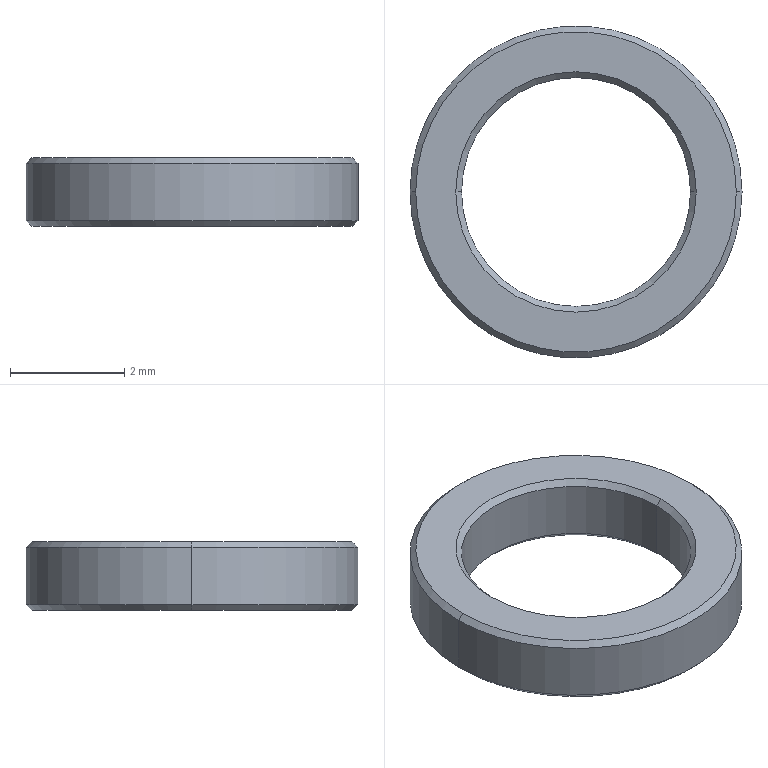Part | SolidWorks | features Revolution 1 | 1 solid | 14 faces | box 5.8 x 5.8 x 1.2 mm | volume 16.317 mm3 | cone 8 | cylinder 4 | plane 2 | commonest cylinder face diameters 4 x2 5.8 x2
STEP:
#1=CARTESIAN_POINT('',(-2.,0.,-1.1));
#2=VERTEX_POINT('',#1);
#3=CARTESIAN_POINT('',(2.,0.,-1.1));
#4=VERTEX_POINT('',#3);
#5=CARTESIAN_POINT('',(0.,0.,-1.1));
#6=DIRECTION('',(0.,0.,1.));
#7=DIRECTION('',(1.,0.,0.));
#8=AXIS2_PLACEMENT_3D('',#5,#6,#7);
#9=CIRCLE('',#8,2.);
#10=EDGE_CURVE('',#2,#4,#9,.T.);
#11=ORIENTED_EDGE('',*,*,#10,.F.);
#12=CARTESIAN_POINT('',(-2.,0.,-0.1));
#13=VERTEX_POINT('',#12);
#14=CARTESIAN_POINT('',(-2.,0.,0.));
#15=DIRECTION('',(0.,0.,1.));
#16=VECTOR('',#15,1000.);
#17=LINE('',#14,#16);
#18=EDGE_CURVE('',#2,#13,#17,.T.);
#19=ORIENTED_EDGE('',*,*,#18,.T.);
#20=CARTESIAN_POINT('',(2.,0.,-0.1));
#21=VERTEX_POINT('',#20);
#22=CARTESIAN_POINT('',(0.,0.,-0.1));
#23=DIRECTION('',(0.,0.,1.));
#24=DIRECTION('',(1.,0.,0.));
#25=AXIS2_PLACEMENT_3D('',#22,#23,#24);
#26=CIRCLE('',#25,2.);
#27=EDGE_CURVE('',#13,#21,#26,.T.);
#28=ORIENTED_EDGE('',*,*,#27,.T.);
#29=CARTESIAN_POINT('',(2.,0.,0.));
#30=DIRECTION('',(0.,0.,1.));
#31=VECTOR('',#30,1000.);
#32=LINE('',#29,#31);
#33=EDGE_CURVE('',#4,#21,#32,.T.);
#34=ORIENTED_EDGE('',*,*,#33,.F.);
#35=EDGE_LOOP('',(#11,#19,#28,#34));
#36=FACE_OUTER_BOUND('',#35,.T.);
#37=CARTESIAN_POINT('',(0.,0.,0.));
#38=DIRECTION('',(0.,0.,1.));
#39=DIRECTION('',(1.,0.,0.));
#40=AXIS2_PLACEMENT_3D('',#37,#38,#39);
#41=CYLINDRICAL_SURFACE('',#40,2.);
#42=ADVANCED_FACE('',(#36),#41,.F.);
#43=ORIENTED_EDGE('',*,*,#10,.T.);
#44=CARTESIAN_POINT('',(2.1,0.,-1.2));
#45=VERTEX_POINT('',#44);
#46=CARTESIAN_POINT('',(2.1,0.,-1.2));
#47=DIRECTION('',(0.7071,0.,-0.7071));
#48=VECTOR('',#47,1000.);
#49=LINE('',#46,#48);
#50=EDGE_CURVE('',#4,#45,#49,.T.);
#51=ORIENTED_EDGE('',*,*,#50,.T.);
#52=CARTESIAN_POINT('',(-2.1,0.,-1.2));
#53=VERTEX_POINT('',#52);
#54=CARTESIAN_POINT('',(0.,0.,-1.2));
#55=DIRECTION('',(0.,0.,1.));
#56=DIRECTION('',(1.,0.,0.));
#57=AXIS2_PLACEMENT_3D('',#54,#55,#56);
#58=CIRCLE('',#57,2.1);
#59=EDGE_CURVE('',#53,#45,#58,.T.);
#60=ORIENTED_EDGE('',*,*,#59,.F.);
#61=CARTESIAN_POINT('',(-2.1,0.,-1.2));
#62=DIRECTION('',(-0.7071,0.,-0.7071));
#63=VECTOR('',#62,1000.);
#64=LINE('',#61,#63);
#65=EDGE_CURVE('',#2,#53,#64,.T.);
#66=ORIENTED_EDGE('',*,*,#65,.F.);
#67=EDGE_LOOP('',(#43,#51,#60,#66));
#68=FACE_OUTER_BOUND('',#67,.T.);
#69=CARTESIAN_POINT('',(0.,0.,-1.2));
#70=DIRECTION('',(0.,0.,-1.));
#71=DIRECTION('',(-1.,0.,0.));
#72=AXIS2_PLACEMENT_3D('',#69,#70,#71);
#73=CONICAL_SURFACE('',#72,2.1,0.7854);
#74=ADVANCED_FACE('',(#68),#73,.F.);
#75=CARTESIAN_POINT('',(2.8,0.,-1.2));
#76=VERTEX_POINT('',#75);
#77=CARTESIAN_POINT('',(-2.8,0.,-1.2));
#78=VERTEX_POINT('',#77);
#79=CARTESIAN_POINT('',(0.,0.,-1.2));
#80=DIRECTION('',(0.,0.,1.));
#81=DIRECTION('',(1.,0.,0.));
#82=AXIS2_PLACEMENT_3D('',#79,#80,#81);
#83=CIRCLE('',#82,2.8);
#84=EDGE_CURVE('',#76,#78,#83,.T.);
#85=ORIENTED_EDGE('',*,*,#84,.T.);
#86=CARTESIAN_POINT('',(-2.9,0.,-1.1));
#87=VERTEX_POINT('',#86);
#88=CARTESIAN_POINT('',(-2.9,0.,-1.1));
#89=DIRECTION('',(-0.7071,0.,0.7071));
#90=VECTOR('',#89,1000.);
#91=LINE('',#88,#90);
#92=EDGE_CURVE('',#78,#87,#91,.T.);
#93=ORIENTED_EDGE('',*,*,#92,.T.);
#94=CARTESIAN_POINT('',(2.9,0.,-1.1));
#95=VERTEX_POINT('',#94);
#96=CARTESIAN_POINT('',(0.,0.,-1.1));
#97=DIRECTION('',(0.,0.,1.));
#98=DIRECTION('',(1.,0.,0.));
#99=AXIS2_PLACEMENT_3D('',#96,#97,#98);
#100=CIRCLE('',#99,2.9);
#101=EDGE_CURVE('',#95,#87,#100,.T.);
#102=ORIENTED_EDGE('',*,*,#101,.F.);
#103=CARTESIAN_POINT('',(2.9,0.,-1.1));
#104=DIRECTION('',(0.7071,0.,0.7071));
#105=VECTOR('',#104,1000.);
#106=LINE('',#103,#105);
#107=EDGE_CURVE('',#76,#95,#106,.T.);
#108=ORIENTED_EDGE('',*,*,#107,.F.);
#109=EDGE_LOOP('',(#85,#93,#102,#108));
#110=FACE_OUTER_BOUND('',#109,.T.);
#111=CARTESIAN_POINT('',(0.,0.,-1.1));
#112=DIRECTION('',(0.,0.,1.));
#113=DIRECTION('',(1.,0.,0.));
#114=AXIS2_PLACEMENT_3D('',#111,#112,#113);
#115=CONICAL_SURFACE('',#114,2.9,0.7854);
#116=ADVANCED_FACE('',(#110),#115,.T.);
#117=ORIENTED_EDGE('',*,*,#101,.T.);
#118=CARTESIAN_POINT('',(-2.9,0.,-0.1));
#119=VERTEX_POINT('',#118);
#120=CARTESIAN_POINT('',(-2.9,0.,0.));
#121=DIRECTION('',(0.,0.,1.));
#122=VECTOR('',#121,1000.);
#123=LINE('',#120,#122);
#124=EDGE_CURVE('',#87,#119,#123,.T.);
#125=ORIENTED_EDGE('',*,*,#124,.T.);
#126=CARTESIAN_POINT('',(2.9,0.,-0.1));
#127=VERTEX_POINT('',#126);
#128=CARTESIAN_POINT('',(0.,0.,-0.1));
#129=DIRECTION('',(0.,0.,1.));
#130=DIRECTION('',(1.,0.,0.));
#131=AXIS2_PLACEMENT_3D('',#128,#129,#130);
#132=CIRCLE('',#131,2.9);
#133=EDGE_CURVE('',#127,#119,#132,.T.);
#134=ORIENTED_EDGE('',*,*,#133,.F.);
#135=CARTESIAN_POINT('',(2.9,0.,0.));
#136=DIRECTION('',(0.,0.,1.));
#137=VECTOR('',#136,1000.);
#138=LINE('',#135,#137);
#139=EDGE_CURVE('',#95,#127,#138,.T.);
#140=ORIENTED_EDGE('',*,*,#139,.F.);
#141=EDGE_LOOP('',(#117,#125,#134,#140));
#142=FACE_OUTER_BOUND('',#141,.T.);
#143=CARTESIAN_POINT('',(0.,0.,0.));
#144=DIRECTION('',(0.,0.,1.));
#145=DIRECTION('',(1.,0.,0.));
#146=AXIS2_PLACEMENT_3D('',#143,#144,#145);
#147=CYLINDRICAL_SURFACE('',#146,2.9);
#148=ADVANCED_FACE('',(#142),#147,.T.);
#149=CARTESIAN_POINT('',(2.8,0.,0.));
#150=VERTEX_POINT('',#149);
#151=CARTESIAN_POINT('',(-2.8,0.,0.));
#152=VERTEX_POINT('',#151);
#153=CARTESIAN_POINT('',(0.,0.,0.));
#154=DIRECTION('',(0.,0.,1.));
#155=DIRECTION('',(1.,0.,0.));
#156=AXIS2_PLACEMENT_3D('',#153,#154,#155);
#157=CIRCLE('',#156,2.8);
#158=EDGE_CURVE('',#150,#152,#157,.T.);
#159=ORIENTED_EDGE('',*,*,#158,.F.);
#160=CARTESIAN_POINT('',(2.8,0.,0.));
#161=DIRECTION('',(0.7071,0.,-0.7071));
#162=VECTOR('',#161,1000.);
#163=LINE('',#160,#162);
#164=EDGE_CURVE('',#150,#127,#163,.T.);
#165=ORIENTED_EDGE('',*,*,#164,.T.);
#166=ORIENTED_EDGE('',*,*,#133,.T.);
#167=CARTESIAN_POINT('',(-2.8,0.,0.));
#168=DIRECTION('',(-0.7071,0.,-0.7071));
#169=VECTOR('',#168,1000.);
#170=LINE('',#167,#169);
#171=EDGE_CURVE('',#152,#119,#170,.T.);
#172=ORIENTED_EDGE('',*,*,#171,.F.);
#173=EDGE_LOOP('',(#159,#165,#166,#172));
#174=FACE_OUTER_BOUND('',#173,.T.);
#175=CARTESIAN_POINT('',(0.,0.,0.));
#176=DIRECTION('',(0.,0.,-1.));
#177=DIRECTION('',(-1.,0.,0.));
#178=AXIS2_PLACEMENT_3D('',#175,#176,#177);
#179=CONICAL_SURFACE('',#178,2.8,0.7854);
#180=ADVANCED_FACE('',(#174),#179,.T.);
#181=ORIENTED_EDGE('',*,*,#27,.F.);
#182=CARTESIAN_POINT('',(-2.1,0.,0.));
#183=VERTEX_POINT('',#182);
#184=CARTESIAN_POINT('',(-2.,0.,-0.1));
#185=DIRECTION('',(-0.7071,0.,0.7071));
#186=VECTOR('',#185,1000.);
#187=LINE('',#184,#186);
#188=EDGE_CURVE('',#13,#183,#187,.T.);
#189=ORIENTED_EDGE('',*,*,#188,.T.);
#190=CARTESIAN_POINT('',(2.1,0.,0.));
#191=VERTEX_POINT('',#190);
#192=CARTESIAN_POINT('',(0.,0.,0.));
#193=DIRECTION('',(0.,0.,1.));
#194=DIRECTION('',(1.,0.,0.));
#195=AXIS2_PLACEMENT_3D('',#192,#193,#194);
#196=CIRCLE('',#195,2.1);
#197=EDGE_CURVE('',#183,#191,#196,.T.);
#198=ORIENTED_EDGE('',*,*,#197,.T.);
#199=CARTESIAN_POINT('',(2.,0.,-0.1));
#200=DIRECTION('',(0.7071,0.,0.7071));
#201=VECTOR('',#200,1000.);
#202=LINE('',#199,#201);
#203=EDGE_CURVE('',#21,#191,#202,.T.);
#204=ORIENTED_EDGE('',*,*,#203,.F.);
#205=EDGE_LOOP('',(#181,#189,#198,#204));
#206=FACE_OUTER_BOUND('',#205,.T.);
#207=CARTESIAN_POINT('',(0.,0.,-0.1));
#208=DIRECTION('',(0.,0.,1.));
#209=DIRECTION('',(1.,0.,0.));
#210=AXIS2_PLACEMENT_3D('',#207,#208,#209);
#211=CONICAL_SURFACE('',#210,2.,0.7854);
#212=ADVANCED_FACE('',(#206),#211,.F.);
#213=ORIENTED_EDGE('',*,*,#188,.F.);
#214=CARTESIAN_POINT('',(0.,0.,-0.1));
#215=DIRECTION('',(0.,0.,1.));
#216=DIRECTION('',(1.,0.,0.));
#217=AXIS2_PLACEMENT_3D('',#214,#215,#216);
#218=CIRCLE('',#217,2.);
#219=EDGE_CURVE('',#21,#13,#218,.T.);
#220=ORIENTED_EDGE('',*,*,#219,.F.);
#221=ORIENTED_EDGE('',*,*,#203,.T.);
#222=CARTESIAN_POINT('',(0.,0.,0.));
#223=DIRECTION('',(0.,0.,1.));
#224=DIRECTION('',(1.,0.,0.));
#225=AXIS2_PLACEMENT_3D('',#222,#223,#224);
#226=CIRCLE('',#225,2.1);
#227=EDGE_CURVE('',#191,#183,#226,.T.);
#228=ORIENTED_EDGE('',*,*,#227,.T.);
#229=EDGE_LOOP('',(#213,#220,#221,#228));
#230=FACE_OUTER_BOUND('',#229,.T.);
#231=CARTESIAN_POINT('',(0.,0.,-0.1));
#232=DIRECTION('',(0.,0.,1.));
#233=DIRECTION('',(1.,0.,0.));
#234=AXIS2_PLACEMENT_3D('',#231,#232,#233);
#235=CONICAL_SURFACE('',#234,2.,0.7854);
#236=ADVANCED_FACE('',(#230),#235,.F.);
#237=CARTESIAN_POINT('',(0.,0.,0.));
#238=DIRECTION('',(0.,0.,1.));
#239=DIRECTION('',(1.,0.,0.));
#240=AXIS2_PLACEMENT_3D('',#237,#238,#239);
#241=CIRCLE('',#240,2.8);
#242=EDGE_CURVE('',#152,#150,#241,.T.);
#243=ORIENTED_EDGE('',*,*,#242,.T.);
#244=ORIENTED_EDGE('',*,*,#158,.T.);
#245=EDGE_LOOP('',(#243,#244));
#246=FACE_OUTER_BOUND('',#245,.T.);
#247=ORIENTED_EDGE('',*,*,#227,.F.);
#248=ORIENTED_EDGE('',*,*,#197,.F.);
#249=EDGE_LOOP('',(#247,#248));
#250=FACE_BOUND('',#249,.T.);
#251=CARTESIAN_POINT('',(2.1,0.,0.));
#252=DIRECTION('',(0.,0.,1.));
#253=DIRECTION('',(1.,0.,0.));
#254=AXIS2_PLACEMENT_3D('',#251,#252,#253);
#255=PLANE('',#254);
#256=ADVANCED_FACE('',(#246,#250),#255,.T.);
#257=ORIENTED_EDGE('',*,*,#164,.F.);
#258=ORIENTED_EDGE('',*,*,#242,.F.);
#259=ORIENTED_EDGE('',*,*,#171,.T.);
#260=CARTESIAN_POINT('',(0.,0.,-0.1));
#261=DIRECTION('',(0.,0.,1.));
#262=DIRECTION('',(1.,0.,0.));
#263=AXIS2_PLACEMENT_3D('',#260,#261,#262);
#264=CIRCLE('',#263,2.9);
#265=EDGE_CURVE('',#119,#127,#264,.T.);
#266=ORIENTED_EDGE('',*,*,#265,.T.);
#267=EDGE_LOOP('',(#257,#258,#259,#266));
#268=FACE_OUTER_BOUND('',#267,.T.);
#269=CARTESIAN_POINT('',(0.,0.,0.));
#270=DIRECTION('',(0.,0.,-1.));
#271=DIRECTION('',(-1.,0.,0.));
#272=AXIS2_PLACEMENT_3D('',#269,#270,#271);
#273=CONICAL_SURFACE('',#272,2.8,0.7854);
#274=ADVANCED_FACE('',(#268),#273,.T.);
#275=ORIENTED_EDGE('',*,*,#124,.F.);
#276=CARTESIAN_POINT('',(0.,0.,-1.1));
#277=DIRECTION('',(0.,0.,1.));
#278=DIRECTION('',(1.,0.,0.));
#279=AXIS2_PLACEMENT_3D('',#276,#277,#278);
#280=CIRCLE('',#279,2.9);
#281=EDGE_CURVE('',#87,#95,#280,.T.);
#282=ORIENTED_EDGE('',*,*,#281,.T.);
#283=ORIENTED_EDGE('',*,*,#139,.T.);
#284=ORIENTED_EDGE('',*,*,#265,.F.);
#285=EDGE_LOOP('',(#275,#282,#283,#284));
#286=FACE_OUTER_BOUND('',#285,.T.);
#287=CARTESIAN_POINT('',(0.,0.,0.));
#288=DIRECTION('',(0.,0.,1.));
#289=DIRECTION('',(1.,0.,0.));
#290=AXIS2_PLACEMENT_3D('',#287,#288,#289);
#291=CYLINDRICAL_SURFACE('',#290,2.9);
#292=ADVANCED_FACE('',(#286),#291,.T.);
#293=ORIENTED_EDGE('',*,*,#92,.F.);
#294=CARTESIAN_POINT('',(0.,0.,-1.2));
#295=DIRECTION('',(0.,0.,1.));
#296=DIRECTION('',(1.,0.,0.));
#297=AXIS2_PLACEMENT_3D('',#294,#295,#296);
#298=CIRCLE('',#297,2.8);
#299=EDGE_CURVE('',#78,#76,#298,.T.);
#300=ORIENTED_EDGE('',*,*,#299,.T.);
#301=ORIENTED_EDGE('',*,*,#107,.T.);
#302=ORIENTED_EDGE('',*,*,#281,.F.);
#303=EDGE_LOOP('',(#293,#300,#301,#302));
#304=FACE_OUTER_BOUND('',#303,.T.);
#305=CARTESIAN_POINT('',(0.,0.,-1.1));
#306=DIRECTION('',(0.,0.,1.));
#307=DIRECTION('',(1.,0.,0.));
#308=AXIS2_PLACEMENT_3D('',#305,#306,#307);
#309=CONICAL_SURFACE('',#308,2.9,0.7854);
#310=ADVANCED_FACE('',(#304),#309,.T.);
#311=ORIENTED_EDGE('',*,*,#59,.T.);
#312=CARTESIAN_POINT('',(0.,0.,-1.2));
#313=DIRECTION('',(0.,0.,1.));
#314=DIRECTION('',(1.,0.,0.));
#315=AXIS2_PLACEMENT_3D('',#312,#313,#314);
#316=CIRCLE('',#315,2.1);
#317=EDGE_CURVE('',#45,#53,#316,.T.);
#318=ORIENTED_EDGE('',*,*,#317,.T.);
#319=EDGE_LOOP('',(#311,#318));
#320=FACE_BOUND('',#319,.T.);
#321=ORIENTED_EDGE('',*,*,#84,.F.);
#322=ORIENTED_EDGE('',*,*,#299,.F.);
#323=EDGE_LOOP('',(#321,#322));
#324=FACE_OUTER_BOUND('',#323,.T.);
#325=CARTESIAN_POINT('',(2.1,0.,-1.2));
#326=DIRECTION('',(0.,0.,-1.));
#327=DIRECTION('',(-1.,0.,0.));
#328=AXIS2_PLACEMENT_3D('',#325,#326,#327);
#329=PLANE('',#328);
#330=ADVANCED_FACE('',(#320,#324),#329,.T.);
#331=ORIENTED_EDGE('',*,*,#50,.F.);
#332=CARTESIAN_POINT('',(0.,0.,-1.1));
#333=DIRECTION('',(0.,0.,1.));
#334=DIRECTION('',(1.,0.,0.));
#335=AXIS2_PLACEMENT_3D('',#332,#333,#334);
#336=CIRCLE('',#335,2.);
#337=EDGE_CURVE('',#4,#2,#336,.T.);
#338=ORIENTED_EDGE('',*,*,#337,.T.);
#339=ORIENTED_EDGE('',*,*,#65,.T.);
#340=ORIENTED_EDGE('',*,*,#317,.F.);
#341=EDGE_LOOP('',(#331,#338,#339,#340));
#342=FACE_OUTER_BOUND('',#341,.T.);
#343=CARTESIAN_POINT('',(0.,0.,-1.2));
#344=DIRECTION('',(0.,0.,-1.));
#345=DIRECTION('',(-1.,0.,0.));
#346=AXIS2_PLACEMENT_3D('',#343,#344,#345);
#347=CONICAL_SURFACE('',#346,2.1,0.7854);
#348=ADVANCED_FACE('',(#342),#347,.F.);
#349=ORIENTED_EDGE('',*,*,#18,.F.);
#350=ORIENTED_EDGE('',*,*,#337,.F.);
#351=ORIENTED_EDGE('',*,*,#33,.T.);
#352=ORIENTED_EDGE('',*,*,#219,.T.);
#353=EDGE_LOOP('',(#349,#350,#351,#352));
#354=FACE_OUTER_BOUND('',#353,.T.);
#355=CARTESIAN_POINT('',(0.,0.,0.));
#356=DIRECTION('',(0.,0.,1.));
#357=DIRECTION('',(1.,0.,0.));
#358=AXIS2_PLACEMENT_3D('',#355,#356,#357);
#359=CYLINDRICAL_SURFACE('',#358,2.);
#360=ADVANCED_FACE('',(#354),#359,.F.);
#361=CLOSED_SHELL('',(#42,#74,#116,#148,#180,#212,#236,#256,#274,#292,#310,#330,#348,#360));
#362=MANIFOLD_SOLID_BREP('',#361);
#363=CARTESIAN_POINT('',(0.,0.,0.));
#364=DIRECTION('',(0.,0.,1.));
#365=DIRECTION('',(1.,0.,0.));
#366=AXIS2_PLACEMENT_3D('',#363,#364,#365);
#367=(LENGTH_UNIT()NAMED_UNIT(*)SI_UNIT(.MILLI.,.METRE.));
#368=UNCERTAINTY_MEASURE_WITH_UNIT(LENGTH_MEASURE(0.00001),#367,'','');
#369=(NAMED_UNIT(*)PLANE_ANGLE_UNIT()SI_UNIT($,.RADIAN.));
#370=(NAMED_UNIT(*)SI_UNIT($,.STERADIAN.)SOLID_ANGLE_UNIT());
#371=(GEOMETRIC_REPRESENTATION_CONTEXT(3)GLOBAL_UNCERTAINTY_ASSIGNED_CONTEXT((#368))GLOBAL_UNIT_ASSIGNED_CONTEXT((#367,#369,#370))REPRESENTATION_CONTEXT('',''));
#372=ADVANCED_BREP_SHAPE_REPRESENTATION('',(#362,#366),#371);